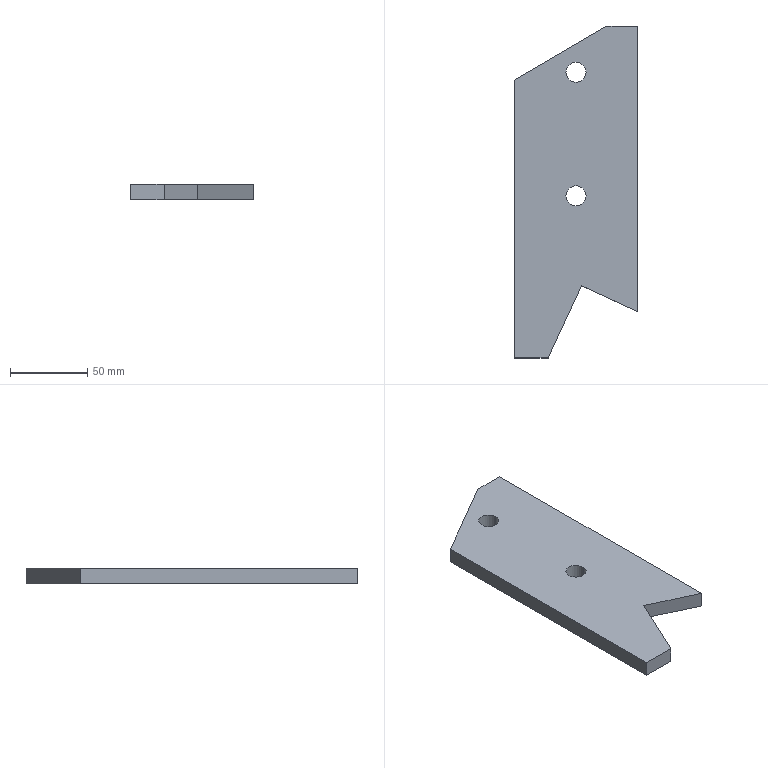Part | SolidWorks | features BaseBody 1 | 1 solid | 13 faces | box 80 x 215 x 10 mm | volume 139823 mm3 | plane 9 | cylinder 4 | commonest cylinder face diameters 13 x4
STEP:
#1=CARTESIAN_POINT('',(-6.5,77.5,0.));
#2=VERTEX_POINT('',#1);
#3=CARTESIAN_POINT('',(6.5,77.5,0.));
#4=VERTEX_POINT('',#3);
#5=CARTESIAN_POINT('',(0.,77.5,0.));
#6=DIRECTION('',(0.,0.,1.));
#7=DIRECTION('',(1.,0.,0.));
#8=AXIS2_PLACEMENT_3D('',#5,#6,#7);
#9=CIRCLE('',#8,6.5);
#10=EDGE_CURVE('',#2,#4,#9,.T.);
#11=ORIENTED_EDGE('',*,*,#10,.F.);
#12=CARTESIAN_POINT('',(-6.5,77.5,10.));
#13=VERTEX_POINT('',#12);
#14=CARTESIAN_POINT('',(-6.5,77.5,0.));
#15=DIRECTION('',(0.,0.,1.));
#16=VECTOR('',#15,1000.);
#17=LINE('',#14,#16);
#18=EDGE_CURVE('',#2,#13,#17,.T.);
#19=ORIENTED_EDGE('',*,*,#18,.T.);
#20=CARTESIAN_POINT('',(6.5,77.5,10.));
#21=VERTEX_POINT('',#20);
#22=CARTESIAN_POINT('',(0.,77.5,10.));
#23=DIRECTION('',(0.,0.,-1.));
#24=DIRECTION('',(1.,0.,0.));
#25=AXIS2_PLACEMENT_3D('',#22,#23,#24);
#26=CIRCLE('',#25,6.5);
#27=EDGE_CURVE('',#21,#13,#26,.T.);
#28=ORIENTED_EDGE('',*,*,#27,.F.);
#29=CARTESIAN_POINT('',(6.5,77.5,0.));
#30=DIRECTION('',(0.,0.,1.));
#31=VECTOR('',#30,1000.);
#32=LINE('',#29,#31);
#33=EDGE_CURVE('',#4,#21,#32,.T.);
#34=ORIENTED_EDGE('',*,*,#33,.F.);
#35=EDGE_LOOP('',(#11,#19,#28,#34));
#36=FACE_OUTER_BOUND('',#35,.T.);
#37=CARTESIAN_POINT('',(0.,77.5,0.));
#38=DIRECTION('',(0.,0.,1.));
#39=DIRECTION('',(1.,0.,0.));
#40=AXIS2_PLACEMENT_3D('',#37,#38,#39);
#41=CYLINDRICAL_SURFACE('',#40,6.5);
#42=ADVANCED_FACE('',(#36),#41,.F.);
#43=CARTESIAN_POINT('',(-6.5,-2.5,0.));
#44=VERTEX_POINT('',#43);
#45=CARTESIAN_POINT('',(6.5,-2.5,0.));
#46=VERTEX_POINT('',#45);
#47=CARTESIAN_POINT('',(0.,-2.5,0.));
#48=DIRECTION('',(0.,0.,1.));
#49=DIRECTION('',(1.,0.,0.));
#50=AXIS2_PLACEMENT_3D('',#47,#48,#49);
#51=CIRCLE('',#50,6.5);
#52=EDGE_CURVE('',#44,#46,#51,.T.);
#53=ORIENTED_EDGE('',*,*,#52,.F.);
#54=CARTESIAN_POINT('',(-6.5,-2.5,10.));
#55=VERTEX_POINT('',#54);
#56=CARTESIAN_POINT('',(-6.5,-2.5,0.));
#57=DIRECTION('',(0.,0.,1.));
#58=VECTOR('',#57,1000.);
#59=LINE('',#56,#58);
#60=EDGE_CURVE('',#44,#55,#59,.T.);
#61=ORIENTED_EDGE('',*,*,#60,.T.);
#62=CARTESIAN_POINT('',(6.5,-2.5,10.));
#63=VERTEX_POINT('',#62);
#64=CARTESIAN_POINT('',(0.,-2.5,10.));
#65=DIRECTION('',(0.,0.,-1.));
#66=DIRECTION('',(1.,0.,0.));
#67=AXIS2_PLACEMENT_3D('',#64,#65,#66);
#68=CIRCLE('',#67,6.5);
#69=EDGE_CURVE('',#63,#55,#68,.T.);
#70=ORIENTED_EDGE('',*,*,#69,.F.);
#71=CARTESIAN_POINT('',(6.5,-2.5,0.));
#72=DIRECTION('',(0.,0.,1.));
#73=VECTOR('',#72,1000.);
#74=LINE('',#71,#73);
#75=EDGE_CURVE('',#46,#63,#74,.T.);
#76=ORIENTED_EDGE('',*,*,#75,.F.);
#77=EDGE_LOOP('',(#53,#61,#70,#76));
#78=FACE_OUTER_BOUND('',#77,.T.);
#79=CARTESIAN_POINT('',(0.,-2.5,0.));
#80=DIRECTION('',(0.,0.,1.));
#81=DIRECTION('',(1.,0.,0.));
#82=AXIS2_PLACEMENT_3D('',#79,#80,#81);
#83=CYLINDRICAL_SURFACE('',#82,6.5);
#84=ADVANCED_FACE('',(#78),#83,.F.);
#85=ORIENTED_EDGE('',*,*,#27,.T.);
#86=CARTESIAN_POINT('',(0.,77.5,10.));
#87=DIRECTION('',(0.,0.,-1.));
#88=DIRECTION('',(1.,0.,0.));
#89=AXIS2_PLACEMENT_3D('',#86,#87,#88);
#90=CIRCLE('',#89,6.5);
#91=EDGE_CURVE('',#13,#21,#90,.T.);
#92=ORIENTED_EDGE('',*,*,#91,.T.);
#93=EDGE_LOOP('',(#85,#92));
#94=FACE_BOUND('',#93,.T.);
#95=ORIENTED_EDGE('',*,*,#69,.T.);
#96=CARTESIAN_POINT('',(0.,-2.5,10.));
#97=DIRECTION('',(0.,0.,-1.));
#98=DIRECTION('',(1.,0.,0.));
#99=AXIS2_PLACEMENT_3D('',#96,#97,#98);
#100=CIRCLE('',#99,6.5);
#101=EDGE_CURVE('',#55,#63,#100,.T.);
#102=ORIENTED_EDGE('',*,*,#101,.T.);
#103=EDGE_LOOP('',(#95,#102));
#104=FACE_BOUND('',#103,.T.);
#105=CARTESIAN_POINT('',(40.,-77.5,10.));
#106=VERTEX_POINT('',#105);
#107=CARTESIAN_POINT('',(40.,107.5,10.));
#108=VERTEX_POINT('',#107);
#109=CARTESIAN_POINT('',(40.,3.212,10.));
#110=DIRECTION('',(0.,1.,0.));
#111=VECTOR('',#110,1000.);
#112=LINE('',#109,#111);
#113=EDGE_CURVE('',#106,#108,#112,.T.);
#114=ORIENTED_EDGE('',*,*,#113,.T.);
#115=CARTESIAN_POINT('',(20.,107.5,10.));
#116=VERTEX_POINT('',#115);
#117=CARTESIAN_POINT('',(-2.245,107.5,10.));
#118=DIRECTION('',(-1.,0.,0.));
#119=VECTOR('',#118,1000.);
#120=LINE('',#117,#119);
#121=EDGE_CURVE('',#108,#116,#120,.T.);
#122=ORIENTED_EDGE('',*,*,#121,.T.);
#123=CARTESIAN_POINT('',(-40.,72.5,10.));
#124=VERTEX_POINT('',#123);
#125=CARTESIAN_POINT('',(20.,107.5,10.));
#126=DIRECTION('',(-0.8638,-0.5039,0.));
#127=VECTOR('',#126,1000.);
#128=LINE('',#125,#127);
#129=EDGE_CURVE('',#116,#124,#128,.T.);
#130=ORIENTED_EDGE('',*,*,#129,.T.);
#131=CARTESIAN_POINT('',(-40.,-107.5,10.));
#132=VERTEX_POINT('',#131);
#133=CARTESIAN_POINT('',(-40.,3.212,10.));
#134=DIRECTION('',(0.,-1.,0.));
#135=VECTOR('',#134,1000.);
#136=LINE('',#133,#135);
#137=EDGE_CURVE('',#124,#132,#136,.T.);
#138=ORIENTED_EDGE('',*,*,#137,.T.);
#139=CARTESIAN_POINT('',(-18.,-107.5,10.));
#140=VERTEX_POINT('',#139);
#141=CARTESIAN_POINT('',(-2.245,-107.5,10.));
#142=DIRECTION('',(1.,0.,0.));
#143=VECTOR('',#142,1000.);
#144=LINE('',#141,#143);
#145=EDGE_CURVE('',#132,#140,#144,.T.);
#146=ORIENTED_EDGE('',*,*,#145,.T.);
#147=CARTESIAN_POINT('',(3.711,-60.674,10.));
#148=VERTEX_POINT('',#147);
#149=CARTESIAN_POINT('',(-18.,-107.5,10.));
#150=DIRECTION('',(0.4206,0.9072,0.));
#151=VECTOR('',#150,1000.);
#152=LINE('',#149,#151);
#153=EDGE_CURVE('',#140,#148,#152,.T.);
#154=ORIENTED_EDGE('',*,*,#153,.T.);
#155=CARTESIAN_POINT('',(3.711,-60.674,10.));
#156=DIRECTION('',(0.9072,-0.4206,0.));
#157=VECTOR('',#156,1000.);
#158=LINE('',#155,#157);
#159=EDGE_CURVE('',#148,#106,#158,.T.);
#160=ORIENTED_EDGE('',*,*,#159,.T.);
#161=EDGE_LOOP('',(#114,#122,#130,#138,#146,#154,#160));
#162=FACE_OUTER_BOUND('',#161,.T.);
#163=CARTESIAN_POINT('',(-2.245,3.212,10.));
#164=DIRECTION('',(0.,0.,1.));
#165=DIRECTION('',(1.,0.,0.));
#166=AXIS2_PLACEMENT_3D('',#163,#164,#165);
#167=PLANE('',#166);
#168=ADVANCED_FACE('',(#94,#104,#162),#167,.T.);
#169=ORIENTED_EDGE('',*,*,#18,.F.);
#170=CARTESIAN_POINT('',(0.,77.5,0.));
#171=DIRECTION('',(0.,0.,1.));
#172=DIRECTION('',(1.,0.,0.));
#173=AXIS2_PLACEMENT_3D('',#170,#171,#172);
#174=CIRCLE('',#173,6.5);
#175=EDGE_CURVE('',#4,#2,#174,.T.);
#176=ORIENTED_EDGE('',*,*,#175,.F.);
#177=ORIENTED_EDGE('',*,*,#33,.T.);
#178=ORIENTED_EDGE('',*,*,#91,.F.);
#179=EDGE_LOOP('',(#169,#176,#177,#178));
#180=FACE_OUTER_BOUND('',#179,.T.);
#181=CARTESIAN_POINT('',(0.,77.5,0.));
#182=DIRECTION('',(0.,0.,1.));
#183=DIRECTION('',(1.,0.,0.));
#184=AXIS2_PLACEMENT_3D('',#181,#182,#183);
#185=CYLINDRICAL_SURFACE('',#184,6.5);
#186=ADVANCED_FACE('',(#180),#185,.F.);
#187=ORIENTED_EDGE('',*,*,#60,.F.);
#188=CARTESIAN_POINT('',(0.,-2.5,0.));
#189=DIRECTION('',(0.,0.,1.));
#190=DIRECTION('',(1.,0.,0.));
#191=AXIS2_PLACEMENT_3D('',#188,#189,#190);
#192=CIRCLE('',#191,6.5);
#193=EDGE_CURVE('',#46,#44,#192,.T.);
#194=ORIENTED_EDGE('',*,*,#193,.F.);
#195=ORIENTED_EDGE('',*,*,#75,.T.);
#196=ORIENTED_EDGE('',*,*,#101,.F.);
#197=EDGE_LOOP('',(#187,#194,#195,#196));
#198=FACE_OUTER_BOUND('',#197,.T.);
#199=CARTESIAN_POINT('',(0.,-2.5,0.));
#200=DIRECTION('',(0.,0.,1.));
#201=DIRECTION('',(1.,0.,0.));
#202=AXIS2_PLACEMENT_3D('',#199,#200,#201);
#203=CYLINDRICAL_SURFACE('',#202,6.5);
#204=ADVANCED_FACE('',(#198),#203,.F.);
#205=CARTESIAN_POINT('',(40.,107.5,0.));
#206=VERTEX_POINT('',#205);
#207=CARTESIAN_POINT('',(40.,107.5,0.));
#208=DIRECTION('',(0.,0.,-1.));
#209=VECTOR('',#208,1000.);
#210=LINE('',#207,#209);
#211=EDGE_CURVE('',#108,#206,#210,.T.);
#212=ORIENTED_EDGE('',*,*,#211,.T.);
#213=CARTESIAN_POINT('',(20.,107.5,0.));
#214=VERTEX_POINT('',#213);
#215=CARTESIAN_POINT('',(-40.,107.5,0.));
#216=DIRECTION('',(-1.,0.,0.));
#217=VECTOR('',#216,1000.);
#218=LINE('',#215,#217);
#219=EDGE_CURVE('',#206,#214,#218,.T.);
#220=ORIENTED_EDGE('',*,*,#219,.T.);
#221=CARTESIAN_POINT('',(20.,107.5,0.));
#222=DIRECTION('',(0.,0.,1.));
#223=VECTOR('',#222,1000.);
#224=LINE('',#221,#223);
#225=EDGE_CURVE('',#214,#116,#224,.T.);
#226=ORIENTED_EDGE('',*,*,#225,.T.);
#227=ORIENTED_EDGE('',*,*,#121,.F.);
#228=EDGE_LOOP('',(#212,#220,#226,#227));
#229=FACE_OUTER_BOUND('',#228,.T.);
#230=CARTESIAN_POINT('',(-40.,107.5,0.));
#231=DIRECTION('',(0.,1.,0.));
#232=DIRECTION('',(-1.,0.,0.));
#233=AXIS2_PLACEMENT_3D('',#230,#231,#232);
#234=PLANE('',#233);
#235=ADVANCED_FACE('',(#229),#234,.T.);
#236=CARTESIAN_POINT('',(40.,-77.5,0.));
#237=VERTEX_POINT('',#236);
#238=CARTESIAN_POINT('',(40.,107.5,0.));
#239=DIRECTION('',(0.,1.,0.));
#240=VECTOR('',#239,1000.);
#241=LINE('',#238,#240);
#242=EDGE_CURVE('',#237,#206,#241,.T.);
#243=ORIENTED_EDGE('',*,*,#242,.T.);
#244=ORIENTED_EDGE('',*,*,#211,.F.);
#245=ORIENTED_EDGE('',*,*,#113,.F.);
#246=CARTESIAN_POINT('',(40.,-77.5,0.));
#247=DIRECTION('',(0.,0.,-1.));
#248=VECTOR('',#247,1000.);
#249=LINE('',#246,#248);
#250=EDGE_CURVE('',#106,#237,#249,.T.);
#251=ORIENTED_EDGE('',*,*,#250,.T.);
#252=EDGE_LOOP('',(#243,#244,#245,#251));
#253=FACE_OUTER_BOUND('',#252,.T.);
#254=CARTESIAN_POINT('',(40.,107.5,0.));
#255=DIRECTION('',(1.,0.,0.));
#256=DIRECTION('',(0.,1.,0.));
#257=AXIS2_PLACEMENT_3D('',#254,#255,#256);
#258=PLANE('',#257);
#259=ADVANCED_FACE('',(#253),#258,.T.);
#260=CARTESIAN_POINT('',(3.711,-60.674,0.));
#261=VERTEX_POINT('',#260);
#262=CARTESIAN_POINT('',(40.,-77.5,0.));
#263=DIRECTION('',(0.9072,-0.4206,0.));
#264=VECTOR('',#263,1000.);
#265=LINE('',#262,#264);
#266=EDGE_CURVE('',#261,#237,#265,.T.);
#267=ORIENTED_EDGE('',*,*,#266,.T.);
#268=ORIENTED_EDGE('',*,*,#250,.F.);
#269=ORIENTED_EDGE('',*,*,#159,.F.);
#270=CARTESIAN_POINT('',(3.711,-60.674,0.));
#271=DIRECTION('',(0.,0.,-1.));
#272=VECTOR('',#271,1000.);
#273=LINE('',#270,#272);
#274=EDGE_CURVE('',#148,#261,#273,.T.);
#275=ORIENTED_EDGE('',*,*,#274,.T.);
#276=EDGE_LOOP('',(#267,#268,#269,#275));
#277=FACE_OUTER_BOUND('',#276,.T.);
#278=CARTESIAN_POINT('',(40.,-77.5,0.));
#279=DIRECTION('',(-0.4206,-0.9072,0.));
#280=DIRECTION('',(0.9072,-0.4206,0.));
#281=AXIS2_PLACEMENT_3D('',#278,#279,#280);
#282=PLANE('',#281);
#283=ADVANCED_FACE('',(#277),#282,.T.);
#284=CARTESIAN_POINT('',(-18.,-107.5,0.));
#285=VERTEX_POINT('',#284);
#286=CARTESIAN_POINT('',(3.711,-60.674,0.));
#287=DIRECTION('',(0.4206,0.9072,0.));
#288=VECTOR('',#287,1000.);
#289=LINE('',#286,#288);
#290=EDGE_CURVE('',#285,#261,#289,.T.);
#291=ORIENTED_EDGE('',*,*,#290,.T.);
#292=ORIENTED_EDGE('',*,*,#274,.F.);
#293=ORIENTED_EDGE('',*,*,#153,.F.);
#294=CARTESIAN_POINT('',(-18.,-107.5,0.));
#295=DIRECTION('',(0.,0.,-1.));
#296=VECTOR('',#295,1000.);
#297=LINE('',#294,#296);
#298=EDGE_CURVE('',#140,#285,#297,.T.);
#299=ORIENTED_EDGE('',*,*,#298,.T.);
#300=EDGE_LOOP('',(#291,#292,#293,#299));
#301=FACE_OUTER_BOUND('',#300,.T.);
#302=CARTESIAN_POINT('',(3.711,-60.674,0.));
#303=DIRECTION('',(0.9072,-0.4206,0.));
#304=DIRECTION('',(0.4206,0.9072,0.));
#305=AXIS2_PLACEMENT_3D('',#302,#303,#304);
#306=PLANE('',#305);
#307=ADVANCED_FACE('',(#301),#306,.T.);
#308=CARTESIAN_POINT('',(-40.,-107.5,0.));
#309=VERTEX_POINT('',#308);
#310=CARTESIAN_POINT('',(-18.,-107.5,0.));
#311=DIRECTION('',(1.,0.,0.));
#312=VECTOR('',#311,1000.);
#313=LINE('',#310,#312);
#314=EDGE_CURVE('',#309,#285,#313,.T.);
#315=ORIENTED_EDGE('',*,*,#314,.T.);
#316=ORIENTED_EDGE('',*,*,#298,.F.);
#317=ORIENTED_EDGE('',*,*,#145,.F.);
#318=CARTESIAN_POINT('',(-40.,-107.5,0.));
#319=DIRECTION('',(0.,0.,-1.));
#320=VECTOR('',#319,1000.);
#321=LINE('',#318,#320);
#322=EDGE_CURVE('',#132,#309,#321,.T.);
#323=ORIENTED_EDGE('',*,*,#322,.T.);
#324=EDGE_LOOP('',(#315,#316,#317,#323));
#325=FACE_OUTER_BOUND('',#324,.T.);
#326=CARTESIAN_POINT('',(-18.,-107.5,0.));
#327=DIRECTION('',(0.,-1.,0.));
#328=DIRECTION('',(1.,0.,0.));
#329=AXIS2_PLACEMENT_3D('',#326,#327,#328);
#330=PLANE('',#329);
#331=ADVANCED_FACE('',(#325),#330,.T.);
#332=ORIENTED_EDGE('',*,*,#322,.F.);
#333=ORIENTED_EDGE('',*,*,#137,.F.);
#334=CARTESIAN_POINT('',(-40.,72.5,0.));
#335=VERTEX_POINT('',#334);
#336=CARTESIAN_POINT('',(-40.,72.5,0.));
#337=DIRECTION('',(0.,0.,-1.));
#338=VECTOR('',#337,1000.);
#339=LINE('',#336,#338);
#340=EDGE_CURVE('',#124,#335,#339,.T.);
#341=ORIENTED_EDGE('',*,*,#340,.T.);
#342=CARTESIAN_POINT('',(-40.,-107.5,0.));
#343=DIRECTION('',(0.,-1.,0.));
#344=VECTOR('',#343,1000.);
#345=LINE('',#342,#344);
#346=EDGE_CURVE('',#335,#309,#345,.T.);
#347=ORIENTED_EDGE('',*,*,#346,.T.);
#348=EDGE_LOOP('',(#332,#333,#341,#347));
#349=FACE_OUTER_BOUND('',#348,.T.);
#350=CARTESIAN_POINT('',(-40.,-107.5,0.));
#351=DIRECTION('',(-1.,0.,0.));
#352=DIRECTION('',(0.,-1.,0.));
#353=AXIS2_PLACEMENT_3D('',#350,#351,#352);
#354=PLANE('',#353);
#355=ADVANCED_FACE('',(#349),#354,.T.);
#356=CARTESIAN_POINT('',(-10.,90.,0.));
#357=DIRECTION('',(-0.8638,-0.5039,0.));
#358=VECTOR('',#357,1000.);
#359=LINE('',#356,#358);
#360=EDGE_CURVE('',#214,#335,#359,.T.);
#361=ORIENTED_EDGE('',*,*,#360,.T.);
#362=ORIENTED_EDGE('',*,*,#340,.F.);
#363=ORIENTED_EDGE('',*,*,#129,.F.);
#364=ORIENTED_EDGE('',*,*,#225,.F.);
#365=EDGE_LOOP('',(#361,#362,#363,#364));
#366=FACE_OUTER_BOUND('',#365,.T.);
#367=CARTESIAN_POINT('',(-10.,90.,0.));
#368=DIRECTION('',(-0.5039,0.8638,0.));
#369=DIRECTION('',(-0.8638,-0.5039,0.));
#370=AXIS2_PLACEMENT_3D('',#367,#368,#369);
#371=PLANE('',#370);
#372=ADVANCED_FACE('',(#366),#371,.T.);
#373=ORIENTED_EDGE('',*,*,#193,.T.);
#374=ORIENTED_EDGE('',*,*,#52,.T.);
#375=EDGE_LOOP('',(#373,#374));
#376=FACE_BOUND('',#375,.T.);
#377=ORIENTED_EDGE('',*,*,#175,.T.);
#378=ORIENTED_EDGE('',*,*,#10,.T.);
#379=EDGE_LOOP('',(#377,#378));
#380=FACE_BOUND('',#379,.T.);
#381=ORIENTED_EDGE('',*,*,#219,.F.);
#382=ORIENTED_EDGE('',*,*,#242,.F.);
#383=ORIENTED_EDGE('',*,*,#266,.F.);
#384=ORIENTED_EDGE('',*,*,#290,.F.);
#385=ORIENTED_EDGE('',*,*,#314,.F.);
#386=ORIENTED_EDGE('',*,*,#346,.F.);
#387=ORIENTED_EDGE('',*,*,#360,.F.);
#388=EDGE_LOOP('',(#381,#382,#383,#384,#385,#386,#387));
#389=FACE_OUTER_BOUND('',#388,.T.);
#390=CARTESIAN_POINT('',(-2.245,3.212,0.));
#391=DIRECTION('',(0.,0.,1.));
#392=DIRECTION('',(1.,0.,0.));
#393=AXIS2_PLACEMENT_3D('',#390,#391,#392);
#394=PLANE('',#393);
#395=ADVANCED_FACE('',(#376,#380,#389),#394,.F.);
#396=CLOSED_SHELL('',(#42,#84,#168,#186,#204,#235,#259,#283,#307,#331,#355,#372,#395));
#397=MANIFOLD_SOLID_BREP('',#396);
#398=CARTESIAN_POINT('',(0.,0.,0.));
#399=DIRECTION('',(0.,0.,1.));
#400=DIRECTION('',(1.,0.,0.));
#401=AXIS2_PLACEMENT_3D('',#398,#399,#400);
#402=(LENGTH_UNIT()NAMED_UNIT(*)SI_UNIT(.MILLI.,.METRE.));
#403=UNCERTAINTY_MEASURE_WITH_UNIT(LENGTH_MEASURE(0.00001),#402,'','');
#404=(NAMED_UNIT(*)PLANE_ANGLE_UNIT()SI_UNIT($,.RADIAN.));
#405=(NAMED_UNIT(*)SI_UNIT($,.STERADIAN.)SOLID_ANGLE_UNIT());
#406=(GEOMETRIC_REPRESENTATION_CONTEXT(3)GLOBAL_UNCERTAINTY_ASSIGNED_CONTEXT((#403))GLOBAL_UNIT_ASSIGNED_CONTEXT((#402,#404,#405))REPRESENTATION_CONTEXT('',''));
#407=ADVANCED_BREP_SHAPE_REPRESENTATION('',(#397,#401),#406);